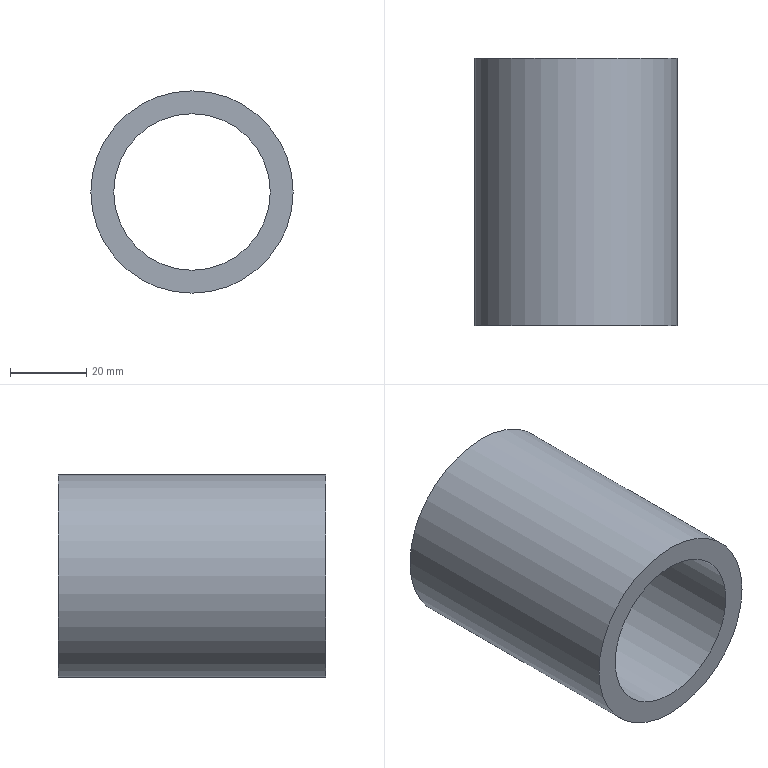Part | NX | features solid 2 | 1 solid | 4 faces | box 53 x 70 x 53 mm | volume 62015 mm3 | plane 2 | cylinder 2 | commonest cylinder face diameters 41 x1 53 x1
STEP:
#1=CARTESIAN_POINT('',(764.5,440.,145.));
#2=VERTEX_POINT('',#1);
#3=CARTESIAN_POINT('',(785.,440.,145.));
#4=DIRECTION('',(0.,-1.,0.));
#5=DIRECTION('',(-1.,0.,0.));
#6=AXIS2_PLACEMENT_3D('',#3,#4,#5);
#7=CIRCLE('',#6,20.5);
#8=EDGE_CURVE('',#2,#2,#7,.F.);
#9=ORIENTED_EDGE('',*,*,#8,.F.);
#10=EDGE_LOOP('',(#9));
#11=FACE_BOUND('',#10,.T.);
#12=CARTESIAN_POINT('',(811.5,440.,145.));
#13=VERTEX_POINT('',#12);
#14=CARTESIAN_POINT('',(785.,440.,145.));
#15=DIRECTION('',(0.,1.,0.));
#16=DIRECTION('',(1.,0.,0.));
#17=AXIS2_PLACEMENT_3D('',#14,#15,#16);
#18=CIRCLE('',#17,26.5);
#19=EDGE_CURVE('',#13,#13,#18,.T.);
#20=ORIENTED_EDGE('',*,*,#19,.T.);
#21=EDGE_LOOP('',(#20));
#22=FACE_BOUND('',#21,.T.);
#23=CARTESIAN_POINT('',(785.,440.,145.));
#24=DIRECTION('',(0.,1.,0.));
#25=DIRECTION('',(-1.,0.,0.));
#26=AXIS2_PLACEMENT_3D('',#23,#24,#25);
#27=PLANE('',#26);
#28=ADVANCED_FACE('',(#11,#22),#27,.T.);
#29=CARTESIAN_POINT('',(764.5,370.,145.));
#30=VERTEX_POINT('',#29);
#31=CARTESIAN_POINT('',(785.,370.,145.));
#32=DIRECTION('',(0.,-1.,0.));
#33=DIRECTION('',(-1.,0.,0.));
#34=AXIS2_PLACEMENT_3D('',#31,#32,#33);
#35=CIRCLE('',#34,20.5);
#36=EDGE_CURVE('',#30,#30,#35,.F.);
#37=ORIENTED_EDGE('',*,*,#36,.T.);
#38=EDGE_LOOP('',(#37));
#39=FACE_BOUND('',#38,.T.);
#40=CARTESIAN_POINT('',(811.5,370.,145.));
#41=VERTEX_POINT('',#40);
#42=CARTESIAN_POINT('',(785.,370.,145.));
#43=DIRECTION('',(0.,1.,0.));
#44=DIRECTION('',(1.,0.,0.));
#45=AXIS2_PLACEMENT_3D('',#42,#43,#44);
#46=CIRCLE('',#45,26.5);
#47=EDGE_CURVE('',#41,#41,#46,.T.);
#48=ORIENTED_EDGE('',*,*,#47,.F.);
#49=EDGE_LOOP('',(#48));
#50=FACE_BOUND('',#49,.T.);
#51=CARTESIAN_POINT('',(785.,370.,145.));
#52=DIRECTION('',(0.,1.,0.));
#53=DIRECTION('',(-1.,0.,0.));
#54=AXIS2_PLACEMENT_3D('',#51,#52,#53);
#55=PLANE('',#54);
#56=ADVANCED_FACE('',(#39,#50),#55,.F.);
#57=ORIENTED_EDGE('',*,*,#8,.T.);
#58=EDGE_LOOP('',(#57));
#59=FACE_BOUND('',#58,.T.);
#60=ORIENTED_EDGE('',*,*,#36,.F.);
#61=EDGE_LOOP('',(#60));
#62=FACE_BOUND('',#61,.T.);
#63=CARTESIAN_POINT('',(785.,370.,145.));
#64=DIRECTION('',(0.,1.,0.));
#65=DIRECTION('',(-1.,0.,0.));
#66=AXIS2_PLACEMENT_3D('',#63,#64,#65);
#67=CYLINDRICAL_SURFACE('',#66,20.5);
#68=ADVANCED_FACE('',(#59,#62),#67,.F.);
#69=ORIENTED_EDGE('',*,*,#19,.F.);
#70=EDGE_LOOP('',(#69));
#71=FACE_BOUND('',#70,.T.);
#72=ORIENTED_EDGE('',*,*,#47,.T.);
#73=EDGE_LOOP('',(#72));
#74=FACE_BOUND('',#73,.T.);
#75=CARTESIAN_POINT('',(785.,370.,145.));
#76=DIRECTION('',(0.,1.,0.));
#77=DIRECTION('',(-1.,0.,0.));
#78=AXIS2_PLACEMENT_3D('',#75,#76,#77);
#79=CYLINDRICAL_SURFACE('',#78,26.5);
#80=ADVANCED_FACE('',(#71,#74),#79,.T.);
#81=CLOSED_SHELL('',(#28,#56,#68,#80));
#82=MANIFOLD_SOLID_BREP('',#81);
#83=(LENGTH_UNIT()NAMED_UNIT(*)SI_UNIT(.MILLI.,.METRE.));
#84=UNCERTAINTY_MEASURE_WITH_UNIT(LENGTH_MEASURE(0.00001),#83,'','');
#85=(NAMED_UNIT(*)PLANE_ANGLE_UNIT()SI_UNIT($,.RADIAN.));
#86=(NAMED_UNIT(*)SI_UNIT($,.STERADIAN.)SOLID_ANGLE_UNIT());
#87=(GEOMETRIC_REPRESENTATION_CONTEXT(3)GLOBAL_UNCERTAINTY_ASSIGNED_CONTEXT((#84))GLOBAL_UNIT_ASSIGNED_CONTEXT((#83,#85,#86))REPRESENTATION_CONTEXT('',''));
#88=ADVANCED_BREP_SHAPE_REPRESENTATION('',(#82),#87);